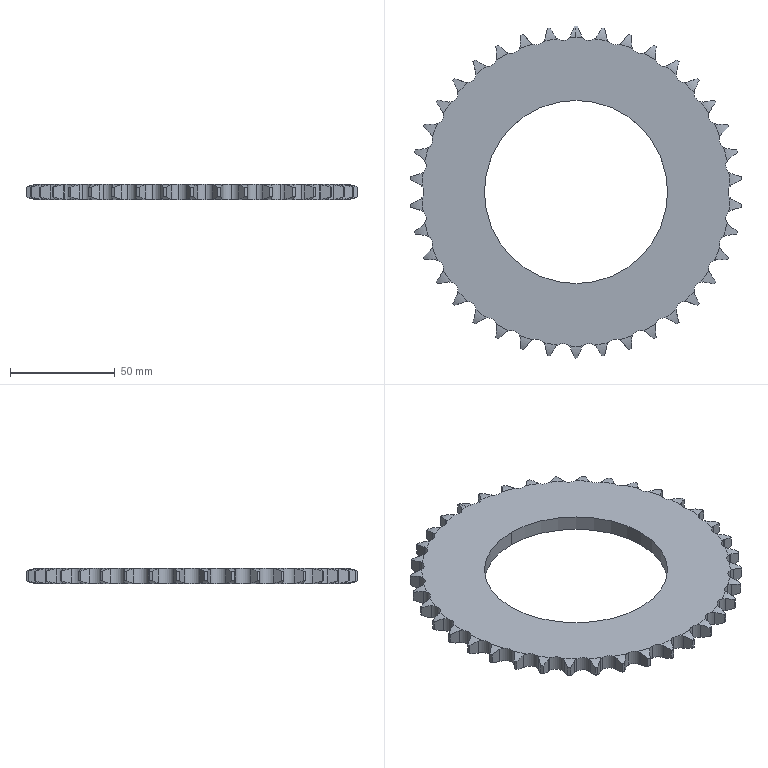Part | SolidWorks | features ICE 5, Revolution 5, CirPattern 3, LPattern 2 | 1 solid | 256 faces | box 158.16 x 158.6 x 7.2 mm | volume 83678 mm3 | cylinder 100 | torus 78 | plane 78 | commonest cylinder face diameters 8.51 x59 158.6 x39 87.5 x2